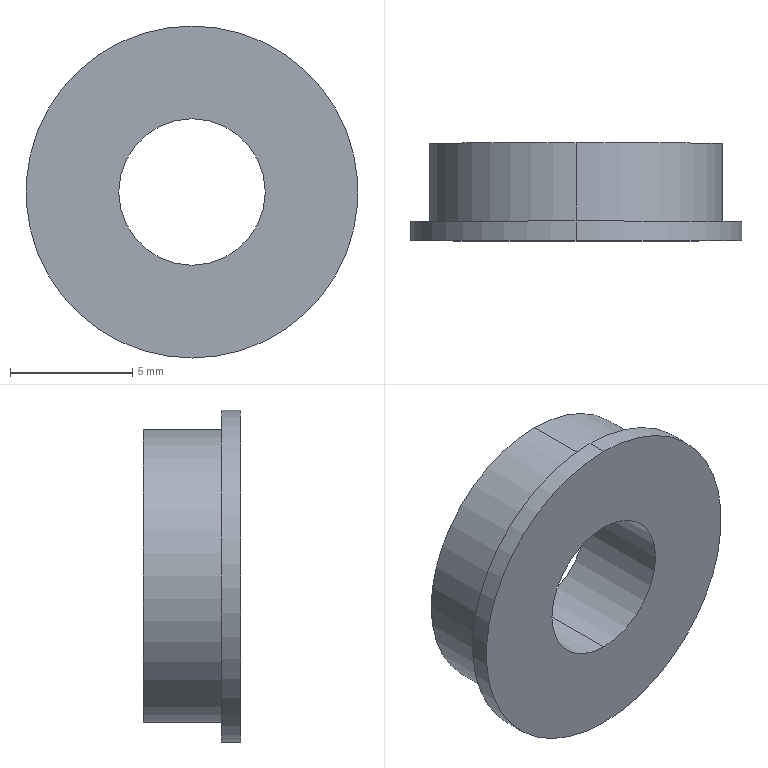Part | SolidWorks | features Extrusion 1, ICE 1 | 1 solid | 9 faces | box 13.6 x 4 x 13.6 mm | volume 365.028 mm3 | cylinder 6 | plane 3 | commonest cylinder face diameters 6 x2 12 x2 13.6 x2
STEP:
#1=CARTESIAN_POINT('',(0.,4.,6.));
#2=VERTEX_POINT('',#1);
#3=CARTESIAN_POINT('',(0.,4.,-6.));
#4=VERTEX_POINT('',#3);
#5=CARTESIAN_POINT('',(0.,4.,0.));
#6=DIRECTION('',(0.,1.,0.));
#7=DIRECTION('',(0.,0.,1.));
#8=AXIS2_PLACEMENT_3D('',#5,#6,#7);
#9=CIRCLE('',#8,6.);
#10=EDGE_CURVE('',#2,#4,#9,.T.);
#11=ORIENTED_EDGE('',*,*,#10,.F.);
#12=CARTESIAN_POINT('',(0.,0.8,6.));
#13=VERTEX_POINT('',#12);
#14=CARTESIAN_POINT('',(0.,4.,6.));
#15=DIRECTION('',(0.,-1.,0.));
#16=VECTOR('',#15,1000.);
#17=LINE('',#14,#16);
#18=EDGE_CURVE('',#2,#13,#17,.T.);
#19=ORIENTED_EDGE('',*,*,#18,.T.);
#20=CARTESIAN_POINT('',(0.,0.8,-6.));
#21=VERTEX_POINT('',#20);
#22=CARTESIAN_POINT('',(0.,0.8,0.));
#23=DIRECTION('',(0.,1.,0.));
#24=DIRECTION('',(0.,0.,1.));
#25=AXIS2_PLACEMENT_3D('',#22,#23,#24);
#26=CIRCLE('',#25,6.);
#27=EDGE_CURVE('',#13,#21,#26,.T.);
#28=ORIENTED_EDGE('',*,*,#27,.T.);
#29=CARTESIAN_POINT('',(0.,4.,-6.));
#30=DIRECTION('',(0.,-1.,0.));
#31=VECTOR('',#30,1000.);
#32=LINE('',#29,#31);
#33=EDGE_CURVE('',#4,#21,#32,.T.);
#34=ORIENTED_EDGE('',*,*,#33,.F.);
#35=EDGE_LOOP('',(#11,#19,#28,#34));
#36=FACE_OUTER_BOUND('',#35,.T.);
#37=CARTESIAN_POINT('',(0.,4.,0.));
#38=DIRECTION('',(0.,-1.,0.));
#39=DIRECTION('',(0.,0.,-1.));
#40=AXIS2_PLACEMENT_3D('',#37,#38,#39);
#41=CYLINDRICAL_SURFACE('',#40,6.);
#42=ADVANCED_FACE('',(#36),#41,.T.);
#43=CARTESIAN_POINT('',(0.,4.,-3.));
#44=VERTEX_POINT('',#43);
#45=CARTESIAN_POINT('',(0.,4.,3.));
#46=VERTEX_POINT('',#45);
#47=CARTESIAN_POINT('',(0.,4.,0.));
#48=DIRECTION('',(0.,1.,0.));
#49=DIRECTION('',(0.,0.,1.));
#50=AXIS2_PLACEMENT_3D('',#47,#48,#49);
#51=CIRCLE('',#50,3.);
#52=EDGE_CURVE('',#44,#46,#51,.T.);
#53=ORIENTED_EDGE('',*,*,#52,.T.);
#54=CARTESIAN_POINT('',(0.,0.,3.));
#55=VERTEX_POINT('',#54);
#56=CARTESIAN_POINT('',(0.,0.8,3.));
#57=DIRECTION('',(0.,-1.,0.));
#58=VECTOR('',#57,1000.);
#59=LINE('',#56,#58);
#60=EDGE_CURVE('',#46,#55,#59,.T.);
#61=ORIENTED_EDGE('',*,*,#60,.T.);
#62=CARTESIAN_POINT('',(0.,0.,-3.));
#63=VERTEX_POINT('',#62);
#64=CARTESIAN_POINT('',(0.,0.,0.));
#65=DIRECTION('',(0.,1.,0.));
#66=DIRECTION('',(0.,0.,1.));
#67=AXIS2_PLACEMENT_3D('',#64,#65,#66);
#68=CIRCLE('',#67,3.);
#69=EDGE_CURVE('',#63,#55,#68,.T.);
#70=ORIENTED_EDGE('',*,*,#69,.F.);
#71=CARTESIAN_POINT('',(0.,0.8,-3.));
#72=DIRECTION('',(0.,-1.,0.));
#73=VECTOR('',#72,1000.);
#74=LINE('',#71,#73);
#75=EDGE_CURVE('',#44,#63,#74,.T.);
#76=ORIENTED_EDGE('',*,*,#75,.F.);
#77=EDGE_LOOP('',(#53,#61,#70,#76));
#78=FACE_OUTER_BOUND('',#77,.T.);
#79=CARTESIAN_POINT('',(0.,0.8,0.));
#80=DIRECTION('',(0.,-1.,0.));
#81=DIRECTION('',(0.,0.,-1.));
#82=AXIS2_PLACEMENT_3D('',#79,#80,#81);
#83=CYLINDRICAL_SURFACE('',#82,3.);
#84=ADVANCED_FACE('',(#78),#83,.F.);
#85=CARTESIAN_POINT('',(0.,0.8,6.8));
#86=VERTEX_POINT('',#85);
#87=CARTESIAN_POINT('',(0.,0.8,-6.8));
#88=VERTEX_POINT('',#87);
#89=CARTESIAN_POINT('',(0.,0.8,0.));
#90=DIRECTION('',(0.,1.,0.));
#91=DIRECTION('',(0.,0.,1.));
#92=AXIS2_PLACEMENT_3D('',#89,#90,#91);
#93=CIRCLE('',#92,6.8);
#94=EDGE_CURVE('',#86,#88,#93,.T.);
#95=ORIENTED_EDGE('',*,*,#94,.F.);
#96=CARTESIAN_POINT('',(0.,0.,6.8));
#97=VERTEX_POINT('',#96);
#98=CARTESIAN_POINT('',(0.,0.8,6.8));
#99=DIRECTION('',(0.,-1.,0.));
#100=VECTOR('',#99,1000.);
#101=LINE('',#98,#100);
#102=EDGE_CURVE('',#86,#97,#101,.T.);
#103=ORIENTED_EDGE('',*,*,#102,.T.);
#104=CARTESIAN_POINT('',(0.,0.,-6.8));
#105=VERTEX_POINT('',#104);
#106=CARTESIAN_POINT('',(0.,0.,0.));
#107=DIRECTION('',(0.,1.,0.));
#108=DIRECTION('',(0.,0.,1.));
#109=AXIS2_PLACEMENT_3D('',#106,#107,#108);
#110=CIRCLE('',#109,6.8);
#111=EDGE_CURVE('',#97,#105,#110,.T.);
#112=ORIENTED_EDGE('',*,*,#111,.T.);
#113=CARTESIAN_POINT('',(0.,0.8,-6.8));
#114=DIRECTION('',(0.,-1.,0.));
#115=VECTOR('',#114,1000.);
#116=LINE('',#113,#115);
#117=EDGE_CURVE('',#88,#105,#116,.T.);
#118=ORIENTED_EDGE('',*,*,#117,.F.);
#119=EDGE_LOOP('',(#95,#103,#112,#118));
#120=FACE_OUTER_BOUND('',#119,.T.);
#121=CARTESIAN_POINT('',(0.,0.8,0.));
#122=DIRECTION('',(0.,-1.,0.));
#123=DIRECTION('',(0.,0.,-1.));
#124=AXIS2_PLACEMENT_3D('',#121,#122,#123);
#125=CYLINDRICAL_SURFACE('',#124,6.8);
#126=ADVANCED_FACE('',(#120),#125,.T.);
#127=CARTESIAN_POINT('',(0.,0.8,0.));
#128=DIRECTION('',(0.,1.,0.));
#129=DIRECTION('',(0.,0.,1.));
#130=AXIS2_PLACEMENT_3D('',#127,#128,#129);
#131=CIRCLE('',#130,6.);
#132=EDGE_CURVE('',#21,#13,#131,.T.);
#133=ORIENTED_EDGE('',*,*,#132,.F.);
#134=ORIENTED_EDGE('',*,*,#27,.F.);
#135=EDGE_LOOP('',(#133,#134));
#136=FACE_BOUND('',#135,.T.);
#137=CARTESIAN_POINT('',(0.,0.8,0.));
#138=DIRECTION('',(0.,1.,0.));
#139=DIRECTION('',(0.,0.,1.));
#140=AXIS2_PLACEMENT_3D('',#137,#138,#139);
#141=CIRCLE('',#140,6.8);
#142=EDGE_CURVE('',#88,#86,#141,.T.);
#143=ORIENTED_EDGE('',*,*,#142,.T.);
#144=ORIENTED_EDGE('',*,*,#94,.T.);
#145=EDGE_LOOP('',(#143,#144));
#146=FACE_OUTER_BOUND('',#145,.T.);
#147=CARTESIAN_POINT('',(0.,0.8,0.));
#148=DIRECTION('',(0.,1.,0.));
#149=DIRECTION('',(0.,0.,1.));
#150=AXIS2_PLACEMENT_3D('',#147,#148,#149);
#151=PLANE('',#150);
#152=ADVANCED_FACE('',(#136,#146),#151,.T.);
#153=CARTESIAN_POINT('',(0.,0.,0.));
#154=DIRECTION('',(0.,1.,0.));
#155=DIRECTION('',(0.,0.,1.));
#156=AXIS2_PLACEMENT_3D('',#153,#154,#155);
#157=CIRCLE('',#156,6.8);
#158=EDGE_CURVE('',#105,#97,#157,.T.);
#159=ORIENTED_EDGE('',*,*,#158,.F.);
#160=ORIENTED_EDGE('',*,*,#111,.F.);
#161=EDGE_LOOP('',(#159,#160));
#162=FACE_OUTER_BOUND('',#161,.T.);
#163=ORIENTED_EDGE('',*,*,#69,.T.);
#164=CARTESIAN_POINT('',(0.,0.,0.));
#165=DIRECTION('',(0.,1.,0.));
#166=DIRECTION('',(0.,0.,1.));
#167=AXIS2_PLACEMENT_3D('',#164,#165,#166);
#168=CIRCLE('',#167,3.);
#169=EDGE_CURVE('',#55,#63,#168,.T.);
#170=ORIENTED_EDGE('',*,*,#169,.T.);
#171=EDGE_LOOP('',(#163,#170));
#172=FACE_BOUND('',#171,.T.);
#173=CARTESIAN_POINT('',(0.,0.,0.));
#174=DIRECTION('',(0.,1.,0.));
#175=DIRECTION('',(0.,0.,1.));
#176=AXIS2_PLACEMENT_3D('',#173,#174,#175);
#177=PLANE('',#176);
#178=ADVANCED_FACE('',(#162,#172),#177,.F.);
#179=ORIENTED_EDGE('',*,*,#102,.F.);
#180=ORIENTED_EDGE('',*,*,#142,.F.);
#181=ORIENTED_EDGE('',*,*,#117,.T.);
#182=ORIENTED_EDGE('',*,*,#158,.T.);
#183=EDGE_LOOP('',(#179,#180,#181,#182));
#184=FACE_OUTER_BOUND('',#183,.T.);
#185=CARTESIAN_POINT('',(0.,0.8,0.));
#186=DIRECTION('',(0.,-1.,0.));
#187=DIRECTION('',(0.,0.,-1.));
#188=AXIS2_PLACEMENT_3D('',#185,#186,#187);
#189=CYLINDRICAL_SURFACE('',#188,6.8);
#190=ADVANCED_FACE('',(#184),#189,.T.);
#191=ORIENTED_EDGE('',*,*,#60,.F.);
#192=CARTESIAN_POINT('',(0.,4.,0.));
#193=DIRECTION('',(0.,1.,0.));
#194=DIRECTION('',(0.,0.,1.));
#195=AXIS2_PLACEMENT_3D('',#192,#193,#194);
#196=CIRCLE('',#195,3.);
#197=EDGE_CURVE('',#46,#44,#196,.T.);
#198=ORIENTED_EDGE('',*,*,#197,.T.);
#199=ORIENTED_EDGE('',*,*,#75,.T.);
#200=ORIENTED_EDGE('',*,*,#169,.F.);
#201=EDGE_LOOP('',(#191,#198,#199,#200));
#202=FACE_OUTER_BOUND('',#201,.T.);
#203=CARTESIAN_POINT('',(0.,0.8,0.));
#204=DIRECTION('',(0.,-1.,0.));
#205=DIRECTION('',(0.,0.,-1.));
#206=AXIS2_PLACEMENT_3D('',#203,#204,#205);
#207=CYLINDRICAL_SURFACE('',#206,3.);
#208=ADVANCED_FACE('',(#202),#207,.F.);
#209=CARTESIAN_POINT('',(0.,4.,0.));
#210=DIRECTION('',(0.,1.,0.));
#211=DIRECTION('',(0.,0.,1.));
#212=AXIS2_PLACEMENT_3D('',#209,#210,#211);
#213=CIRCLE('',#212,6.);
#214=EDGE_CURVE('',#4,#2,#213,.T.);
#215=ORIENTED_EDGE('',*,*,#214,.T.);
#216=ORIENTED_EDGE('',*,*,#10,.T.);
#217=EDGE_LOOP('',(#215,#216));
#218=FACE_OUTER_BOUND('',#217,.T.);
#219=ORIENTED_EDGE('',*,*,#52,.F.);
#220=ORIENTED_EDGE('',*,*,#197,.F.);
#221=EDGE_LOOP('',(#219,#220));
#222=FACE_BOUND('',#221,.T.);
#223=CARTESIAN_POINT('',(0.,4.,0.));
#224=DIRECTION('',(0.,1.,0.));
#225=DIRECTION('',(0.,0.,1.));
#226=AXIS2_PLACEMENT_3D('',#223,#224,#225);
#227=PLANE('',#226);
#228=ADVANCED_FACE('',(#218,#222),#227,.T.);
#229=ORIENTED_EDGE('',*,*,#18,.F.);
#230=ORIENTED_EDGE('',*,*,#214,.F.);
#231=ORIENTED_EDGE('',*,*,#33,.T.);
#232=ORIENTED_EDGE('',*,*,#132,.T.);
#233=EDGE_LOOP('',(#229,#230,#231,#232));
#234=FACE_OUTER_BOUND('',#233,.T.);
#235=CARTESIAN_POINT('',(0.,4.,0.));
#236=DIRECTION('',(0.,-1.,0.));
#237=DIRECTION('',(0.,0.,-1.));
#238=AXIS2_PLACEMENT_3D('',#235,#236,#237);
#239=CYLINDRICAL_SURFACE('',#238,6.);
#240=ADVANCED_FACE('',(#234),#239,.T.);
#241=CLOSED_SHELL('',(#42,#84,#126,#152,#178,#190,#208,#228,#240));
#242=MANIFOLD_SOLID_BREP('',#241);
#243=CARTESIAN_POINT('',(0.,0.,0.));
#244=DIRECTION('',(0.,0.,1.));
#245=DIRECTION('',(1.,0.,0.));
#246=AXIS2_PLACEMENT_3D('',#243,#244,#245);
#247=(LENGTH_UNIT()NAMED_UNIT(*)SI_UNIT(.MILLI.,.METRE.));
#248=UNCERTAINTY_MEASURE_WITH_UNIT(LENGTH_MEASURE(0.00001),#247,'','');
#249=(NAMED_UNIT(*)PLANE_ANGLE_UNIT()SI_UNIT($,.RADIAN.));
#250=(NAMED_UNIT(*)SI_UNIT($,.STERADIAN.)SOLID_ANGLE_UNIT());
#251=(GEOMETRIC_REPRESENTATION_CONTEXT(3)GLOBAL_UNCERTAINTY_ASSIGNED_CONTEXT((#248))GLOBAL_UNIT_ASSIGNED_CONTEXT((#247,#249,#250))REPRESENTATION_CONTEXT('',''));
#252=ADVANCED_BREP_SHAPE_REPRESENTATION('',(#242,#246),#251);